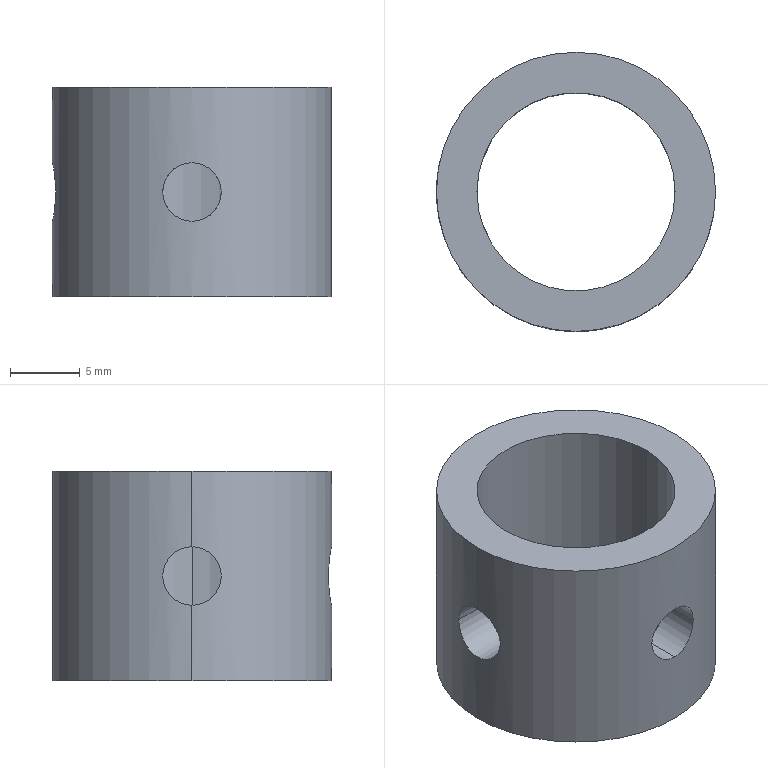Part | STEP file | 1 solid | 10 faces | box 20 x 20 x 15 mm | volume 2256 mm3 | cylinder 8 | plane 2 | commonest cylinder face diameters 4.2 x4 14.2 x2 20 x2